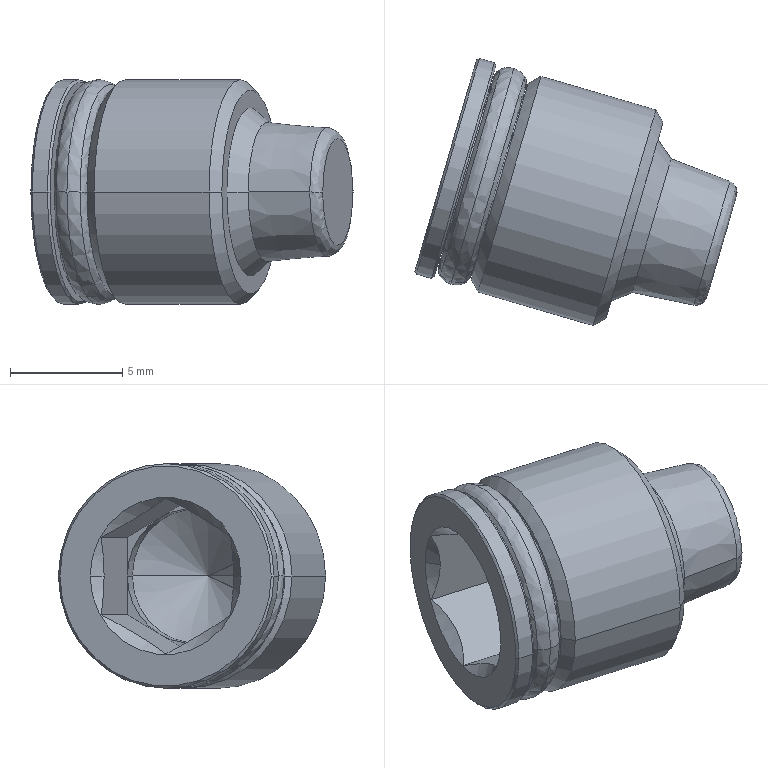Part | SolidWorks | features BaseBody 1 | 1 solid | 57 faces | box 14.343 x 11.893 x 10 mm | volume 615.272 mm3 | plane 17 | cone 16 | spline 14 | cylinder 10 | commonest cylinder face diameters 7.7 x4 10 x4 6 x2